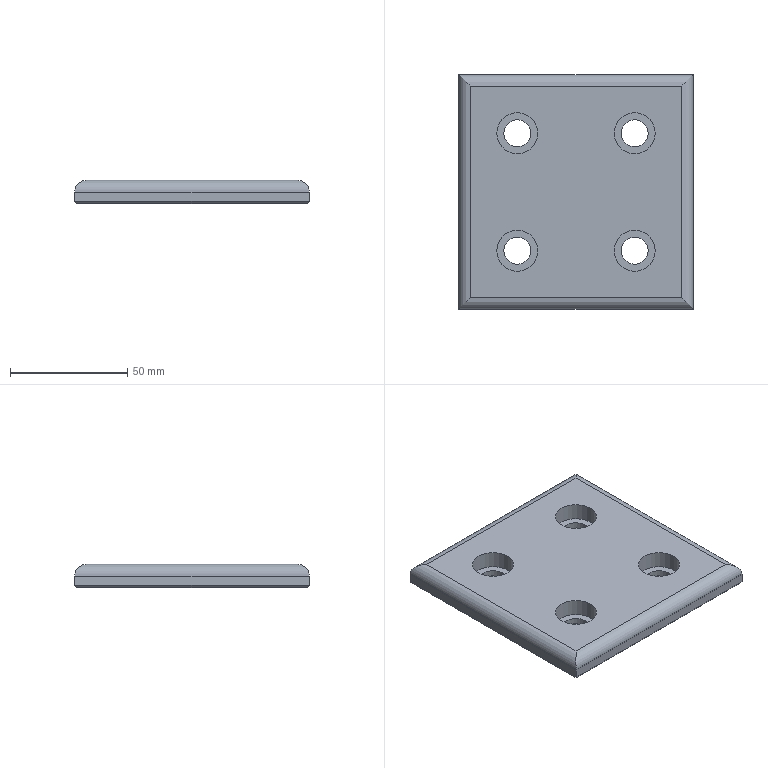Part | NX | features solid 2 | 1 solid | 26 faces | box 100 x 100 x 10 mm | volume 89558 mm3 | plane 14 | cylinder 12 | commonest cylinder face diameters 10 x4 11.5 x4 17.5 x4
STEP:
#1=CARTESIAN_POINT('',(-480.,-730.,-129.));
#2=VERTEX_POINT('',#1);
#3=CARTESIAN_POINT('',(-480.,-730.,-125.));
#4=VERTEX_POINT('',#3);
#5=CARTESIAN_POINT('',(-480.,-730.,-130.));
#6=DIRECTION('',(0.,0.,1.));
#7=VECTOR('',#6,1000.);
#8=LINE('',#5,#7);
#9=EDGE_CURVE('',#2,#4,#8,.T.);
#10=ORIENTED_EDGE('',*,*,#9,.T.);
#11=CARTESIAN_POINT('',(-480.,-630.,-125.));
#12=VERTEX_POINT('',#11);
#13=CARTESIAN_POINT('',(-480.,-730.,-125.));
#14=DIRECTION('',(0.,-1.,0.));
#15=VECTOR('',#14,1000.);
#16=LINE('',#13,#15);
#17=EDGE_CURVE('',#12,#4,#16,.T.);
#18=ORIENTED_EDGE('',*,*,#17,.F.);
#19=CARTESIAN_POINT('',(-480.,-630.,-129.));
#20=VERTEX_POINT('',#19);
#21=CARTESIAN_POINT('',(-480.,-630.,-130.));
#22=DIRECTION('',(0.,0.,1.));
#23=VECTOR('',#22,1000.);
#24=LINE('',#21,#23);
#25=EDGE_CURVE('',#20,#12,#24,.T.);
#26=ORIENTED_EDGE('',*,*,#25,.F.);
#27=CARTESIAN_POINT('',(-480.,-630.,-129.));
#28=DIRECTION('',(0.,1.,0.));
#29=VECTOR('',#28,1000.);
#30=LINE('',#27,#29);
#31=EDGE_CURVE('',#2,#20,#30,.T.);
#32=ORIENTED_EDGE('',*,*,#31,.F.);
#33=EDGE_LOOP('',(#10,#18,#26,#32));
#34=FACE_BOUND('',#33,.T.);
#35=CARTESIAN_POINT('',(-480.,-630.,-130.));
#36=DIRECTION('',(1.,0.,0.));
#37=DIRECTION('',(0.,-1.,0.));
#38=AXIS2_PLACEMENT_3D('',#35,#36,#37);
#39=PLANE('',#38);
#40=ADVANCED_FACE('',(#34),#39,.F.);
#41=CARTESIAN_POINT('',(-380.,-730.,-129.));
#42=VERTEX_POINT('',#41);
#43=CARTESIAN_POINT('',(-380.,-730.,-125.));
#44=VERTEX_POINT('',#43);
#45=CARTESIAN_POINT('',(-380.,-730.,-130.));
#46=DIRECTION('',(0.,0.,1.));
#47=VECTOR('',#46,1000.);
#48=LINE('',#45,#47);
#49=EDGE_CURVE('',#42,#44,#48,.T.);
#50=ORIENTED_EDGE('',*,*,#49,.T.);
#51=CARTESIAN_POINT('',(-380.,-730.,-125.));
#52=DIRECTION('',(1.,0.,0.));
#53=VECTOR('',#52,1000.);
#54=LINE('',#51,#53);
#55=EDGE_CURVE('',#4,#44,#54,.T.);
#56=ORIENTED_EDGE('',*,*,#55,.F.);
#57=ORIENTED_EDGE('',*,*,#9,.F.);
#58=CARTESIAN_POINT('',(-530.,-730.,-129.));
#59=DIRECTION('',(-1.,0.,0.));
#60=VECTOR('',#59,1000.);
#61=LINE('',#58,#60);
#62=EDGE_CURVE('',#42,#2,#61,.T.);
#63=ORIENTED_EDGE('',*,*,#62,.F.);
#64=EDGE_LOOP('',(#50,#56,#57,#63));
#65=FACE_BOUND('',#64,.T.);
#66=CARTESIAN_POINT('',(-530.,-730.,-130.));
#67=DIRECTION('',(0.,1.,0.));
#68=DIRECTION('',(1.,0.,0.));
#69=AXIS2_PLACEMENT_3D('',#66,#67,#68);
#70=PLANE('',#69);
#71=ADVANCED_FACE('',(#65),#70,.F.);
#72=CARTESIAN_POINT('',(-380.,-630.,-129.));
#73=VERTEX_POINT('',#72);
#74=CARTESIAN_POINT('',(-380.,-630.,-125.));
#75=VERTEX_POINT('',#74);
#76=CARTESIAN_POINT('',(-380.,-630.,-130.));
#77=DIRECTION('',(0.,0.,1.));
#78=VECTOR('',#77,1000.);
#79=LINE('',#76,#78);
#80=EDGE_CURVE('',#73,#75,#79,.T.);
#81=ORIENTED_EDGE('',*,*,#80,.T.);
#82=CARTESIAN_POINT('',(-380.,-630.,-125.));
#83=DIRECTION('',(0.,1.,0.));
#84=VECTOR('',#83,1000.);
#85=LINE('',#82,#84);
#86=EDGE_CURVE('',#44,#75,#85,.T.);
#87=ORIENTED_EDGE('',*,*,#86,.F.);
#88=ORIENTED_EDGE('',*,*,#49,.F.);
#89=CARTESIAN_POINT('',(-380.,-730.,-129.));
#90=DIRECTION('',(0.,-1.,0.));
#91=VECTOR('',#90,1000.);
#92=LINE('',#89,#91);
#93=EDGE_CURVE('',#73,#42,#92,.T.);
#94=ORIENTED_EDGE('',*,*,#93,.F.);
#95=EDGE_LOOP('',(#81,#87,#88,#94));
#96=FACE_BOUND('',#95,.T.);
#97=CARTESIAN_POINT('',(-380.,-730.,-130.));
#98=DIRECTION('',(-1.,0.,0.));
#99=DIRECTION('',(0.,1.,0.));
#100=AXIS2_PLACEMENT_3D('',#97,#98,#99);
#101=PLANE('',#100);
#102=ADVANCED_FACE('',(#96),#101,.F.);
#103=ORIENTED_EDGE('',*,*,#25,.T.);
#104=CARTESIAN_POINT('',(-530.,-630.,-125.));
#105=DIRECTION('',(-1.,0.,0.));
#106=VECTOR('',#105,1000.);
#107=LINE('',#104,#106);
#108=EDGE_CURVE('',#75,#12,#107,.T.);
#109=ORIENTED_EDGE('',*,*,#108,.F.);
#110=ORIENTED_EDGE('',*,*,#80,.F.);
#111=CARTESIAN_POINT('',(-380.,-630.,-129.));
#112=DIRECTION('',(1.,0.,0.));
#113=VECTOR('',#112,1000.);
#114=LINE('',#111,#113);
#115=EDGE_CURVE('',#20,#73,#114,.T.);
#116=ORIENTED_EDGE('',*,*,#115,.F.);
#117=EDGE_LOOP('',(#103,#109,#110,#116));
#118=FACE_BOUND('',#117,.T.);
#119=CARTESIAN_POINT('',(-380.,-630.,-130.));
#120=DIRECTION('',(0.,-1.,0.));
#121=DIRECTION('',(-1.,0.,0.));
#122=AXIS2_PLACEMENT_3D('',#119,#120,#121);
#123=PLANE('',#122);
#124=ADVANCED_FACE('',(#118),#123,.F.);
#125=CARTESIAN_POINT('',(-479.,-631.,-130.));
#126=VERTEX_POINT('',#125);
#127=CARTESIAN_POINT('',(-479.,-729.,-130.));
#128=VERTEX_POINT('',#127);
#129=CARTESIAN_POINT('',(-479.,-630.,-130.));
#130=DIRECTION('',(0.,1.,0.));
#131=VECTOR('',#130,1000.);
#132=LINE('',#129,#131);
#133=EDGE_CURVE('',#126,#128,#132,.F.);
#134=ORIENTED_EDGE('',*,*,#133,.F.);
#135=CARTESIAN_POINT('',(-381.,-631.,-130.));
#136=VERTEX_POINT('',#135);
#137=CARTESIAN_POINT('',(-530.,-631.,-130.));
#138=DIRECTION('',(-1.,0.,0.));
#139=VECTOR('',#138,1000.);
#140=LINE('',#137,#139);
#141=EDGE_CURVE('',#136,#126,#140,.T.);
#142=ORIENTED_EDGE('',*,*,#141,.F.);
#143=CARTESIAN_POINT('',(-381.,-729.,-130.));
#144=VERTEX_POINT('',#143);
#145=CARTESIAN_POINT('',(-381.,-630.,-130.));
#146=DIRECTION('',(0.,1.,0.));
#147=VECTOR('',#146,1000.);
#148=LINE('',#145,#147);
#149=EDGE_CURVE('',#144,#136,#148,.T.);
#150=ORIENTED_EDGE('',*,*,#149,.F.);
#151=CARTESIAN_POINT('',(-530.,-729.,-130.));
#152=DIRECTION('',(1.,0.,0.));
#153=VECTOR('',#152,1000.);
#154=LINE('',#151,#153);
#155=EDGE_CURVE('',#128,#144,#154,.T.);
#156=ORIENTED_EDGE('',*,*,#155,.F.);
#157=EDGE_LOOP('',(#134,#142,#150,#156));
#158=FACE_BOUND('',#157,.T.);
#159=CARTESIAN_POINT('',(-399.25,-655.,-130.));
#160=VERTEX_POINT('',#159);
#161=CARTESIAN_POINT('',(-405.,-655.,-130.));
#162=DIRECTION('',(0.,0.,-1.));
#163=DIRECTION('',(1.,0.,0.));
#164=AXIS2_PLACEMENT_3D('',#161,#162,#163);
#165=CIRCLE('',#164,5.75);
#166=EDGE_CURVE('',#160,#160,#165,.T.);
#167=ORIENTED_EDGE('',*,*,#166,.F.);
#168=EDGE_LOOP('',(#167));
#169=FACE_BOUND('',#168,.T.);
#170=CARTESIAN_POINT('',(-399.25,-705.,-130.));
#171=VERTEX_POINT('',#170);
#172=CARTESIAN_POINT('',(-405.,-705.,-130.));
#173=DIRECTION('',(0.,0.,-1.));
#174=DIRECTION('',(1.,0.,0.));
#175=AXIS2_PLACEMENT_3D('',#172,#173,#174);
#176=CIRCLE('',#175,5.75);
#177=EDGE_CURVE('',#171,#171,#176,.T.);
#178=ORIENTED_EDGE('',*,*,#177,.F.);
#179=EDGE_LOOP('',(#178));
#180=FACE_BOUND('',#179,.T.);
#181=CARTESIAN_POINT('',(-460.75,-655.,-130.));
#182=VERTEX_POINT('',#181);
#183=CARTESIAN_POINT('',(-455.,-655.,-130.));
#184=DIRECTION('',(0.,0.,-1.));
#185=DIRECTION('',(-1.,0.,0.));
#186=AXIS2_PLACEMENT_3D('',#183,#184,#185);
#187=CIRCLE('',#186,5.75);
#188=EDGE_CURVE('',#182,#182,#187,.T.);
#189=ORIENTED_EDGE('',*,*,#188,.F.);
#190=EDGE_LOOP('',(#189));
#191=FACE_BOUND('',#190,.T.);
#192=CARTESIAN_POINT('',(-460.75,-705.,-130.));
#193=VERTEX_POINT('',#192);
#194=CARTESIAN_POINT('',(-455.,-705.,-130.));
#195=DIRECTION('',(0.,0.,-1.));
#196=DIRECTION('',(-1.,0.,0.));
#197=AXIS2_PLACEMENT_3D('',#194,#195,#196);
#198=CIRCLE('',#197,5.75);
#199=EDGE_CURVE('',#193,#193,#198,.T.);
#200=ORIENTED_EDGE('',*,*,#199,.F.);
#201=EDGE_LOOP('',(#200));
#202=FACE_BOUND('',#201,.T.);
#203=CARTESIAN_POINT('',(-530.,-630.,-130.));
#204=DIRECTION('',(0.,0.,1.));
#205=DIRECTION('',(1.,0.,0.));
#206=AXIS2_PLACEMENT_3D('',#203,#204,#205);
#207=PLANE('',#206);
#208=ADVANCED_FACE('',(#158,#169,#180,#191,#202),#207,.F.);
#209=CARTESIAN_POINT('',(-385.,-635.,-120.));
#210=VERTEX_POINT('',#209);
#211=CARTESIAN_POINT('',(-385.,-725.,-120.));
#212=VERTEX_POINT('',#211);
#213=CARTESIAN_POINT('',(-385.,-730.,-120.));
#214=DIRECTION('',(0.,1.,0.));
#215=VECTOR('',#214,1000.);
#216=LINE('',#213,#215);
#217=EDGE_CURVE('',#210,#212,#216,.F.);
#218=ORIENTED_EDGE('',*,*,#217,.F.);
#219=CARTESIAN_POINT('',(-475.,-635.,-120.));
#220=VERTEX_POINT('',#219);
#221=CARTESIAN_POINT('',(-380.,-635.,-120.));
#222=DIRECTION('',(-1.,0.,0.));
#223=VECTOR('',#222,1000.);
#224=LINE('',#221,#223);
#225=EDGE_CURVE('',#220,#210,#224,.F.);
#226=ORIENTED_EDGE('',*,*,#225,.F.);
#227=CARTESIAN_POINT('',(-475.,-725.,-120.));
#228=VERTEX_POINT('',#227);
#229=CARTESIAN_POINT('',(-475.,-630.,-120.));
#230=DIRECTION('',(0.,-1.,0.));
#231=VECTOR('',#230,1000.);
#232=LINE('',#229,#231);
#233=EDGE_CURVE('',#228,#220,#232,.F.);
#234=ORIENTED_EDGE('',*,*,#233,.F.);
#235=CARTESIAN_POINT('',(-530.,-725.,-120.));
#236=DIRECTION('',(1.,0.,0.));
#237=VECTOR('',#236,1000.);
#238=LINE('',#235,#237);
#239=EDGE_CURVE('',#212,#228,#238,.F.);
#240=ORIENTED_EDGE('',*,*,#239,.F.);
#241=EDGE_LOOP('',(#218,#226,#234,#240));
#242=FACE_BOUND('',#241,.T.);
#243=CARTESIAN_POINT('',(-413.75,-655.,-120.));
#244=VERTEX_POINT('',#243);
#245=CARTESIAN_POINT('',(-405.,-655.,-120.));
#246=DIRECTION('',(0.,0.,1.));
#247=DIRECTION('',(-1.,0.,0.));
#248=AXIS2_PLACEMENT_3D('',#245,#246,#247);
#249=CIRCLE('',#248,8.75);
#250=EDGE_CURVE('',#244,#244,#249,.T.);
#251=ORIENTED_EDGE('',*,*,#250,.F.);
#252=EDGE_LOOP('',(#251));
#253=FACE_BOUND('',#252,.T.);
#254=CARTESIAN_POINT('',(-413.75,-705.,-120.));
#255=VERTEX_POINT('',#254);
#256=CARTESIAN_POINT('',(-405.,-705.,-120.));
#257=DIRECTION('',(0.,0.,1.));
#258=DIRECTION('',(-1.,0.,0.));
#259=AXIS2_PLACEMENT_3D('',#256,#257,#258);
#260=CIRCLE('',#259,8.75);
#261=EDGE_CURVE('',#255,#255,#260,.T.);
#262=ORIENTED_EDGE('',*,*,#261,.F.);
#263=EDGE_LOOP('',(#262));
#264=FACE_BOUND('',#263,.T.);
#265=CARTESIAN_POINT('',(-463.75,-655.,-120.));
#266=VERTEX_POINT('',#265);
#267=CARTESIAN_POINT('',(-455.,-655.,-120.));
#268=DIRECTION('',(0.,0.,-1.));
#269=DIRECTION('',(-1.,0.,0.));
#270=AXIS2_PLACEMENT_3D('',#267,#268,#269);
#271=CIRCLE('',#270,8.75);
#272=EDGE_CURVE('',#266,#266,#271,.F.);
#273=ORIENTED_EDGE('',*,*,#272,.F.);
#274=EDGE_LOOP('',(#273));
#275=FACE_BOUND('',#274,.T.);
#276=CARTESIAN_POINT('',(-463.75,-705.,-120.));
#277=VERTEX_POINT('',#276);
#278=CARTESIAN_POINT('',(-455.,-705.,-120.));
#279=DIRECTION('',(0.,0.,-1.));
#280=DIRECTION('',(-1.,0.,0.));
#281=AXIS2_PLACEMENT_3D('',#278,#279,#280);
#282=CIRCLE('',#281,8.75);
#283=EDGE_CURVE('',#277,#277,#282,.F.);
#284=ORIENTED_EDGE('',*,*,#283,.F.);
#285=EDGE_LOOP('',(#284));
#286=FACE_BOUND('',#285,.T.);
#287=CARTESIAN_POINT('',(-530.,-630.,-120.));
#288=DIRECTION('',(0.,0.,1.));
#289=DIRECTION('',(1.,0.,0.));
#290=AXIS2_PLACEMENT_3D('',#287,#288,#289);
#291=PLANE('',#290);
#292=ADVANCED_FACE('',(#242,#253,#264,#275,#286),#291,.T.);
#293=CARTESIAN_POINT('',(-460.75,-705.,-127.3));
#294=VERTEX_POINT('',#293);
#295=CARTESIAN_POINT('',(-455.,-705.,-127.3));
#296=DIRECTION('',(0.,0.,1.));
#297=DIRECTION('',(-1.,0.,0.));
#298=AXIS2_PLACEMENT_3D('',#295,#296,#297);
#299=CIRCLE('',#298,5.75);
#300=EDGE_CURVE('',#294,#294,#299,.T.);
#301=ORIENTED_EDGE('',*,*,#300,.T.);
#302=EDGE_LOOP('',(#301));
#303=FACE_BOUND('',#302,.T.);
#304=ORIENTED_EDGE('',*,*,#199,.T.);
#305=EDGE_LOOP('',(#304));
#306=FACE_BOUND('',#305,.T.);
#307=CARTESIAN_POINT('',(-455.,-705.,-170.));
#308=DIRECTION('',(0.,0.,-1.));
#309=DIRECTION('',(-1.,0.,0.));
#310=AXIS2_PLACEMENT_3D('',#307,#308,#309);
#311=CYLINDRICAL_SURFACE('',#310,5.75);
#312=ADVANCED_FACE('',(#303,#306),#311,.F.);
#313=ORIENTED_EDGE('',*,*,#300,.F.);
#314=EDGE_LOOP('',(#313));
#315=FACE_BOUND('',#314,.T.);
#316=CARTESIAN_POINT('',(-463.75,-705.,-127.3));
#317=VERTEX_POINT('',#316);
#318=CARTESIAN_POINT('',(-455.,-705.,-127.3));
#319=DIRECTION('',(0.,0.,1.));
#320=DIRECTION('',(-1.,0.,0.));
#321=AXIS2_PLACEMENT_3D('',#318,#319,#320);
#322=CIRCLE('',#321,8.75);
#323=EDGE_CURVE('',#317,#317,#322,.T.);
#324=ORIENTED_EDGE('',*,*,#323,.T.);
#325=EDGE_LOOP('',(#324));
#326=FACE_BOUND('',#325,.T.);
#327=CARTESIAN_POINT('',(-455.,-705.,-127.3));
#328=DIRECTION('',(0.,0.,-1.));
#329=DIRECTION('',(-1.,0.,0.));
#330=AXIS2_PLACEMENT_3D('',#327,#328,#329);
#331=PLANE('',#330);
#332=ADVANCED_FACE('',(#315,#326),#331,.F.);
#333=ORIENTED_EDGE('',*,*,#323,.F.);
#334=EDGE_LOOP('',(#333));
#335=FACE_BOUND('',#334,.T.);
#336=ORIENTED_EDGE('',*,*,#283,.T.);
#337=EDGE_LOOP('',(#336));
#338=FACE_BOUND('',#337,.T.);
#339=CARTESIAN_POINT('',(-455.,-705.,-120.));
#340=DIRECTION('',(0.,0.,-1.));
#341=DIRECTION('',(-1.,0.,0.));
#342=AXIS2_PLACEMENT_3D('',#339,#340,#341);
#343=CYLINDRICAL_SURFACE('',#342,8.75);
#344=ADVANCED_FACE('',(#335,#338),#343,.F.);
#345=CARTESIAN_POINT('',(-460.75,-655.,-127.3));
#346=VERTEX_POINT('',#345);
#347=CARTESIAN_POINT('',(-455.,-655.,-127.3));
#348=DIRECTION('',(0.,0.,1.));
#349=DIRECTION('',(-1.,0.,0.));
#350=AXIS2_PLACEMENT_3D('',#347,#348,#349);
#351=CIRCLE('',#350,5.75);
#352=EDGE_CURVE('',#346,#346,#351,.T.);
#353=ORIENTED_EDGE('',*,*,#352,.T.);
#354=EDGE_LOOP('',(#353));
#355=FACE_BOUND('',#354,.T.);
#356=ORIENTED_EDGE('',*,*,#188,.T.);
#357=EDGE_LOOP('',(#356));
#358=FACE_BOUND('',#357,.T.);
#359=CARTESIAN_POINT('',(-455.,-655.,-170.));
#360=DIRECTION('',(0.,0.,-1.));
#361=DIRECTION('',(-1.,0.,0.));
#362=AXIS2_PLACEMENT_3D('',#359,#360,#361);
#363=CYLINDRICAL_SURFACE('',#362,5.75);
#364=ADVANCED_FACE('',(#355,#358),#363,.F.);
#365=ORIENTED_EDGE('',*,*,#352,.F.);
#366=EDGE_LOOP('',(#365));
#367=FACE_BOUND('',#366,.T.);
#368=CARTESIAN_POINT('',(-463.75,-655.,-127.3));
#369=VERTEX_POINT('',#368);
#370=CARTESIAN_POINT('',(-455.,-655.,-127.3));
#371=DIRECTION('',(0.,0.,1.));
#372=DIRECTION('',(-1.,0.,0.));
#373=AXIS2_PLACEMENT_3D('',#370,#371,#372);
#374=CIRCLE('',#373,8.75);
#375=EDGE_CURVE('',#369,#369,#374,.T.);
#376=ORIENTED_EDGE('',*,*,#375,.T.);
#377=EDGE_LOOP('',(#376));
#378=FACE_BOUND('',#377,.T.);
#379=CARTESIAN_POINT('',(-455.,-655.,-127.3));
#380=DIRECTION('',(0.,0.,-1.));
#381=DIRECTION('',(-1.,0.,0.));
#382=AXIS2_PLACEMENT_3D('',#379,#380,#381);
#383=PLANE('',#382);
#384=ADVANCED_FACE('',(#367,#378),#383,.F.);
#385=ORIENTED_EDGE('',*,*,#375,.F.);
#386=EDGE_LOOP('',(#385));
#387=FACE_BOUND('',#386,.T.);
#388=ORIENTED_EDGE('',*,*,#272,.T.);
#389=EDGE_LOOP('',(#388));
#390=FACE_BOUND('',#389,.T.);
#391=CARTESIAN_POINT('',(-455.,-655.,-120.));
#392=DIRECTION('',(0.,0.,-1.));
#393=DIRECTION('',(-1.,0.,0.));
#394=AXIS2_PLACEMENT_3D('',#391,#392,#393);
#395=CYLINDRICAL_SURFACE('',#394,8.75);
#396=ADVANCED_FACE('',(#387,#390),#395,.F.);
#397=CARTESIAN_POINT('',(-410.75,-705.,-127.3));
#398=VERTEX_POINT('',#397);
#399=CARTESIAN_POINT('',(-405.,-705.,-127.3));
#400=DIRECTION('',(0.,0.,1.));
#401=DIRECTION('',(-1.,0.,0.));
#402=AXIS2_PLACEMENT_3D('',#399,#400,#401);
#403=CIRCLE('',#402,5.75);
#404=EDGE_CURVE('',#398,#398,#403,.T.);
#405=ORIENTED_EDGE('',*,*,#404,.T.);
#406=EDGE_LOOP('',(#405));
#407=FACE_BOUND('',#406,.T.);
#408=ORIENTED_EDGE('',*,*,#177,.T.);
#409=EDGE_LOOP('',(#408));
#410=FACE_BOUND('',#409,.T.);
#411=CARTESIAN_POINT('',(-405.,-705.,-170.));
#412=DIRECTION('',(0.,0.,-1.));
#413=DIRECTION('',(-1.,0.,0.));
#414=AXIS2_PLACEMENT_3D('',#411,#412,#413);
#415=CYLINDRICAL_SURFACE('',#414,5.75);
#416=ADVANCED_FACE('',(#407,#410),#415,.F.);
#417=ORIENTED_EDGE('',*,*,#404,.F.);
#418=EDGE_LOOP('',(#417));
#419=FACE_BOUND('',#418,.T.);
#420=CARTESIAN_POINT('',(-413.75,-705.,-127.3));
#421=VERTEX_POINT('',#420);
#422=CARTESIAN_POINT('',(-405.,-705.,-127.3));
#423=DIRECTION('',(0.,0.,1.));
#424=DIRECTION('',(-1.,0.,0.));
#425=AXIS2_PLACEMENT_3D('',#422,#423,#424);
#426=CIRCLE('',#425,8.75);
#427=EDGE_CURVE('',#421,#421,#426,.T.);
#428=ORIENTED_EDGE('',*,*,#427,.T.);
#429=EDGE_LOOP('',(#428));
#430=FACE_BOUND('',#429,.T.);
#431=CARTESIAN_POINT('',(-405.,-705.,-127.3));
#432=DIRECTION('',(0.,0.,-1.));
#433=DIRECTION('',(-1.,0.,0.));
#434=AXIS2_PLACEMENT_3D('',#431,#432,#433);
#435=PLANE('',#434);
#436=ADVANCED_FACE('',(#419,#430),#435,.F.);
#437=ORIENTED_EDGE('',*,*,#427,.F.);
#438=EDGE_LOOP('',(#437));
#439=FACE_BOUND('',#438,.T.);
#440=ORIENTED_EDGE('',*,*,#261,.T.);
#441=EDGE_LOOP('',(#440));
#442=FACE_BOUND('',#441,.T.);
#443=CARTESIAN_POINT('',(-405.,-705.,-120.));
#444=DIRECTION('',(0.,0.,-1.));
#445=DIRECTION('',(-1.,0.,0.));
#446=AXIS2_PLACEMENT_3D('',#443,#444,#445);
#447=CYLINDRICAL_SURFACE('',#446,8.75);
#448=ADVANCED_FACE('',(#439,#442),#447,.F.);
#449=CARTESIAN_POINT('',(-410.75,-655.,-127.3));
#450=VERTEX_POINT('',#449);
#451=CARTESIAN_POINT('',(-405.,-655.,-127.3));
#452=DIRECTION('',(0.,0.,1.));
#453=DIRECTION('',(-1.,0.,0.));
#454=AXIS2_PLACEMENT_3D('',#451,#452,#453);
#455=CIRCLE('',#454,5.75);
#456=EDGE_CURVE('',#450,#450,#455,.T.);
#457=ORIENTED_EDGE('',*,*,#456,.T.);
#458=EDGE_LOOP('',(#457));
#459=FACE_BOUND('',#458,.T.);
#460=ORIENTED_EDGE('',*,*,#166,.T.);
#461=EDGE_LOOP('',(#460));
#462=FACE_BOUND('',#461,.T.);
#463=CARTESIAN_POINT('',(-405.,-655.,-170.));
#464=DIRECTION('',(0.,0.,-1.));
#465=DIRECTION('',(-1.,0.,0.));
#466=AXIS2_PLACEMENT_3D('',#463,#464,#465);
#467=CYLINDRICAL_SURFACE('',#466,5.75);
#468=ADVANCED_FACE('',(#459,#462),#467,.F.);
#469=ORIENTED_EDGE('',*,*,#456,.F.);
#470=EDGE_LOOP('',(#469));
#471=FACE_BOUND('',#470,.T.);
#472=CARTESIAN_POINT('',(-413.75,-655.,-127.3));
#473=VERTEX_POINT('',#472);
#474=CARTESIAN_POINT('',(-405.,-655.,-127.3));
#475=DIRECTION('',(0.,0.,1.));
#476=DIRECTION('',(-1.,0.,0.));
#477=AXIS2_PLACEMENT_3D('',#474,#475,#476);
#478=CIRCLE('',#477,8.75);
#479=EDGE_CURVE('',#473,#473,#478,.T.);
#480=ORIENTED_EDGE('',*,*,#479,.T.);
#481=EDGE_LOOP('',(#480));
#482=FACE_BOUND('',#481,.T.);
#483=CARTESIAN_POINT('',(-405.,-655.,-127.3));
#484=DIRECTION('',(0.,0.,-1.));
#485=DIRECTION('',(-1.,0.,0.));
#486=AXIS2_PLACEMENT_3D('',#483,#484,#485);
#487=PLANE('',#486);
#488=ADVANCED_FACE('',(#471,#482),#487,.F.);
#489=ORIENTED_EDGE('',*,*,#479,.F.);
#490=EDGE_LOOP('',(#489));
#491=FACE_BOUND('',#490,.T.);
#492=ORIENTED_EDGE('',*,*,#250,.T.);
#493=EDGE_LOOP('',(#492));
#494=FACE_BOUND('',#493,.T.);
#495=CARTESIAN_POINT('',(-405.,-655.,-120.));
#496=DIRECTION('',(0.,0.,-1.));
#497=DIRECTION('',(-1.,0.,0.));
#498=AXIS2_PLACEMENT_3D('',#495,#496,#497);
#499=CYLINDRICAL_SURFACE('',#498,8.75);
#500=ADVANCED_FACE('',(#491,#494),#499,.F.);
#501=CARTESIAN_POINT('',(-385.,-635.,-125.));
#502=DIRECTION('',(-0.7071,0.7071,0.));
#503=DIRECTION('',(0.7071,0.7071,0.));
#504=AXIS2_PLACEMENT_3D('',#501,#502,#503);
#505=ELLIPSE('',#504,7.071,5.);
#506=EDGE_CURVE('',#210,#75,#505,.T.);
#507=ORIENTED_EDGE('',*,*,#506,.T.);
#508=ORIENTED_EDGE('',*,*,#108,.T.);
#509=CARTESIAN_POINT('',(-475.,-635.,-125.));
#510=DIRECTION('',(-0.7071,-0.7071,0.));
#511=DIRECTION('',(-0.7071,0.7071,0.));
#512=AXIS2_PLACEMENT_3D('',#509,#510,#511);
#513=ELLIPSE('',#512,7.071,5.);
#514=EDGE_CURVE('',#12,#220,#513,.F.);
#515=ORIENTED_EDGE('',*,*,#514,.T.);
#516=ORIENTED_EDGE('',*,*,#225,.T.);
#517=EDGE_LOOP('',(#507,#508,#515,#516));
#518=FACE_BOUND('',#517,.T.);
#519=CARTESIAN_POINT('',(-380.,-635.,-125.));
#520=DIRECTION('',(1.,0.,0.));
#521=DIRECTION('',(0.,-1.,0.));
#522=AXIS2_PLACEMENT_3D('',#519,#520,#521);
#523=CYLINDRICAL_SURFACE('',#522,5.);
#524=ADVANCED_FACE('',(#518),#523,.T.);
#525=ORIENTED_EDGE('',*,*,#514,.F.);
#526=ORIENTED_EDGE('',*,*,#17,.T.);
#527=CARTESIAN_POINT('',(-475.,-725.,-125.));
#528=DIRECTION('',(0.7071,-0.7071,0.));
#529=DIRECTION('',(-0.7071,-0.7071,0.));
#530=AXIS2_PLACEMENT_3D('',#527,#528,#529);
#531=ELLIPSE('',#530,7.071,5.);
#532=EDGE_CURVE('',#4,#228,#531,.F.);
#533=ORIENTED_EDGE('',*,*,#532,.T.);
#534=ORIENTED_EDGE('',*,*,#233,.T.);
#535=EDGE_LOOP('',(#525,#526,#533,#534));
#536=FACE_BOUND('',#535,.T.);
#537=CARTESIAN_POINT('',(-475.,-630.,-125.));
#538=DIRECTION('',(0.,1.,0.));
#539=DIRECTION('',(1.,0.,0.));
#540=AXIS2_PLACEMENT_3D('',#537,#538,#539);
#541=CYLINDRICAL_SURFACE('',#540,5.);
#542=ADVANCED_FACE('',(#536),#541,.T.);
#543=ORIENTED_EDGE('',*,*,#506,.F.);
#544=ORIENTED_EDGE('',*,*,#217,.T.);
#545=CARTESIAN_POINT('',(-385.,-725.,-125.));
#546=DIRECTION('',(0.7071,0.7071,0.));
#547=DIRECTION('',(0.7071,-0.7071,0.));
#548=AXIS2_PLACEMENT_3D('',#545,#546,#547);
#549=ELLIPSE('',#548,7.071,5.);
#550=EDGE_CURVE('',#212,#44,#549,.T.);
#551=ORIENTED_EDGE('',*,*,#550,.T.);
#552=ORIENTED_EDGE('',*,*,#86,.T.);
#553=EDGE_LOOP('',(#543,#544,#551,#552));
#554=FACE_BOUND('',#553,.T.);
#555=CARTESIAN_POINT('',(-385.,-730.,-125.));
#556=DIRECTION('',(0.,-1.,0.));
#557=DIRECTION('',(-1.,0.,0.));
#558=AXIS2_PLACEMENT_3D('',#555,#556,#557);
#559=CYLINDRICAL_SURFACE('',#558,5.);
#560=ADVANCED_FACE('',(#554),#559,.T.);
#561=ORIENTED_EDGE('',*,*,#532,.F.);
#562=ORIENTED_EDGE('',*,*,#55,.T.);
#563=ORIENTED_EDGE('',*,*,#550,.F.);
#564=ORIENTED_EDGE('',*,*,#239,.T.);
#565=EDGE_LOOP('',(#561,#562,#563,#564));
#566=FACE_BOUND('',#565,.T.);
#567=CARTESIAN_POINT('',(-530.,-725.,-125.));
#568=DIRECTION('',(-1.,0.,0.));
#569=DIRECTION('',(0.,1.,0.));
#570=AXIS2_PLACEMENT_3D('',#567,#568,#569);
#571=CYLINDRICAL_SURFACE('',#570,5.);
#572=ADVANCED_FACE('',(#566),#571,.T.);
#573=CARTESIAN_POINT('',(-430.667,-680.667,-179.667));
#574=DIRECTION('',(0.5774,0.5774,0.5774));
#575=VECTOR('',#574,1000.);
#576=LINE('',#573,#575);
#577=EDGE_CURVE('',#73,#136,#576,.F.);
#578=ORIENTED_EDGE('',*,*,#577,.T.);
#579=ORIENTED_EDGE('',*,*,#141,.T.);
#580=CARTESIAN_POINT('',(-479.333,-630.667,-129.667));
#581=DIRECTION('',(-0.5774,0.5774,0.5774));
#582=VECTOR('',#581,1000.);
#583=LINE('',#580,#582);
#584=EDGE_CURVE('',#126,#20,#583,.T.);
#585=ORIENTED_EDGE('',*,*,#584,.T.);
#586=ORIENTED_EDGE('',*,*,#115,.T.);
#587=EDGE_LOOP('',(#578,#579,#585,#586));
#588=FACE_BOUND('',#587,.T.);
#589=CARTESIAN_POINT('',(-530.,-631.,-130.));
#590=DIRECTION('',(0.,-0.7071,0.7071));
#591=DIRECTION('',(0.,0.7071,0.7071));
#592=AXIS2_PLACEMENT_3D('',#589,#590,#591);
#593=PLANE('',#592);
#594=ADVANCED_FACE('',(#588),#593,.F.);
#595=ORIENTED_EDGE('',*,*,#584,.F.);
#596=ORIENTED_EDGE('',*,*,#133,.T.);
#597=CARTESIAN_POINT('',(-496.,-746.,-113.));
#598=DIRECTION('',(-0.5774,-0.5774,0.5774));
#599=VECTOR('',#598,1000.);
#600=LINE('',#597,#599);
#601=EDGE_CURVE('',#128,#2,#600,.T.);
#602=ORIENTED_EDGE('',*,*,#601,.T.);
#603=ORIENTED_EDGE('',*,*,#31,.T.);
#604=EDGE_LOOP('',(#595,#596,#602,#603));
#605=FACE_BOUND('',#604,.T.);
#606=CARTESIAN_POINT('',(-479.,-630.,-130.));
#607=DIRECTION('',(0.7071,0.,0.7071));
#608=DIRECTION('',(0.7071,0.,-0.7071));
#609=AXIS2_PLACEMENT_3D('',#606,#607,#608);
#610=PLANE('',#609);
#611=ADVANCED_FACE('',(#605),#610,.F.);
#612=ORIENTED_EDGE('',*,*,#577,.F.);
#613=ORIENTED_EDGE('',*,*,#93,.T.);
#614=CARTESIAN_POINT('',(-414.,-696.,-163.));
#615=DIRECTION('',(0.5774,-0.5774,0.5774));
#616=VECTOR('',#615,1000.);
#617=LINE('',#614,#616);
#618=EDGE_CURVE('',#42,#144,#617,.F.);
#619=ORIENTED_EDGE('',*,*,#618,.T.);
#620=ORIENTED_EDGE('',*,*,#149,.T.);
#621=EDGE_LOOP('',(#612,#613,#619,#620));
#622=FACE_BOUND('',#621,.T.);
#623=CARTESIAN_POINT('',(-381.,-630.,-130.));
#624=DIRECTION('',(-0.7071,0.,0.7071));
#625=DIRECTION('',(0.7071,0.,0.7071));
#626=AXIS2_PLACEMENT_3D('',#623,#624,#625);
#627=PLANE('',#626);
#628=ADVANCED_FACE('',(#622),#627,.F.);
#629=ORIENTED_EDGE('',*,*,#601,.F.);
#630=ORIENTED_EDGE('',*,*,#155,.T.);
#631=ORIENTED_EDGE('',*,*,#618,.F.);
#632=ORIENTED_EDGE('',*,*,#62,.T.);
#633=EDGE_LOOP('',(#629,#630,#631,#632));
#634=FACE_BOUND('',#633,.T.);
#635=CARTESIAN_POINT('',(-530.,-729.,-130.));
#636=DIRECTION('',(0.,0.7071,0.7071));
#637=DIRECTION('',(0.,0.7071,-0.7071));
#638=AXIS2_PLACEMENT_3D('',#635,#636,#637);
#639=PLANE('',#638);
#640=ADVANCED_FACE('',(#634),#639,.F.);
#641=CLOSED_SHELL('',(#40,#71,#102,#124,#208,#292,#312,#332,#344,#364,#384,#396,#416,#436,#448,#468,#488,#500,#524,#542,#560,#572,#594,#611,#628,#640));
#642=MANIFOLD_SOLID_BREP('',#641);
#643=(LENGTH_UNIT()NAMED_UNIT(*)SI_UNIT(.MILLI.,.METRE.));
#644=UNCERTAINTY_MEASURE_WITH_UNIT(LENGTH_MEASURE(0.00001),#643,'','');
#645=(NAMED_UNIT(*)PLANE_ANGLE_UNIT()SI_UNIT($,.RADIAN.));
#646=(NAMED_UNIT(*)SI_UNIT($,.STERADIAN.)SOLID_ANGLE_UNIT());
#647=(GEOMETRIC_REPRESENTATION_CONTEXT(3)GLOBAL_UNCERTAINTY_ASSIGNED_CONTEXT((#644))GLOBAL_UNIT_ASSIGNED_CONTEXT((#643,#645,#646))REPRESENTATION_CONTEXT('',''));
#648=ADVANCED_BREP_SHAPE_REPRESENTATION('',(#642),#647);